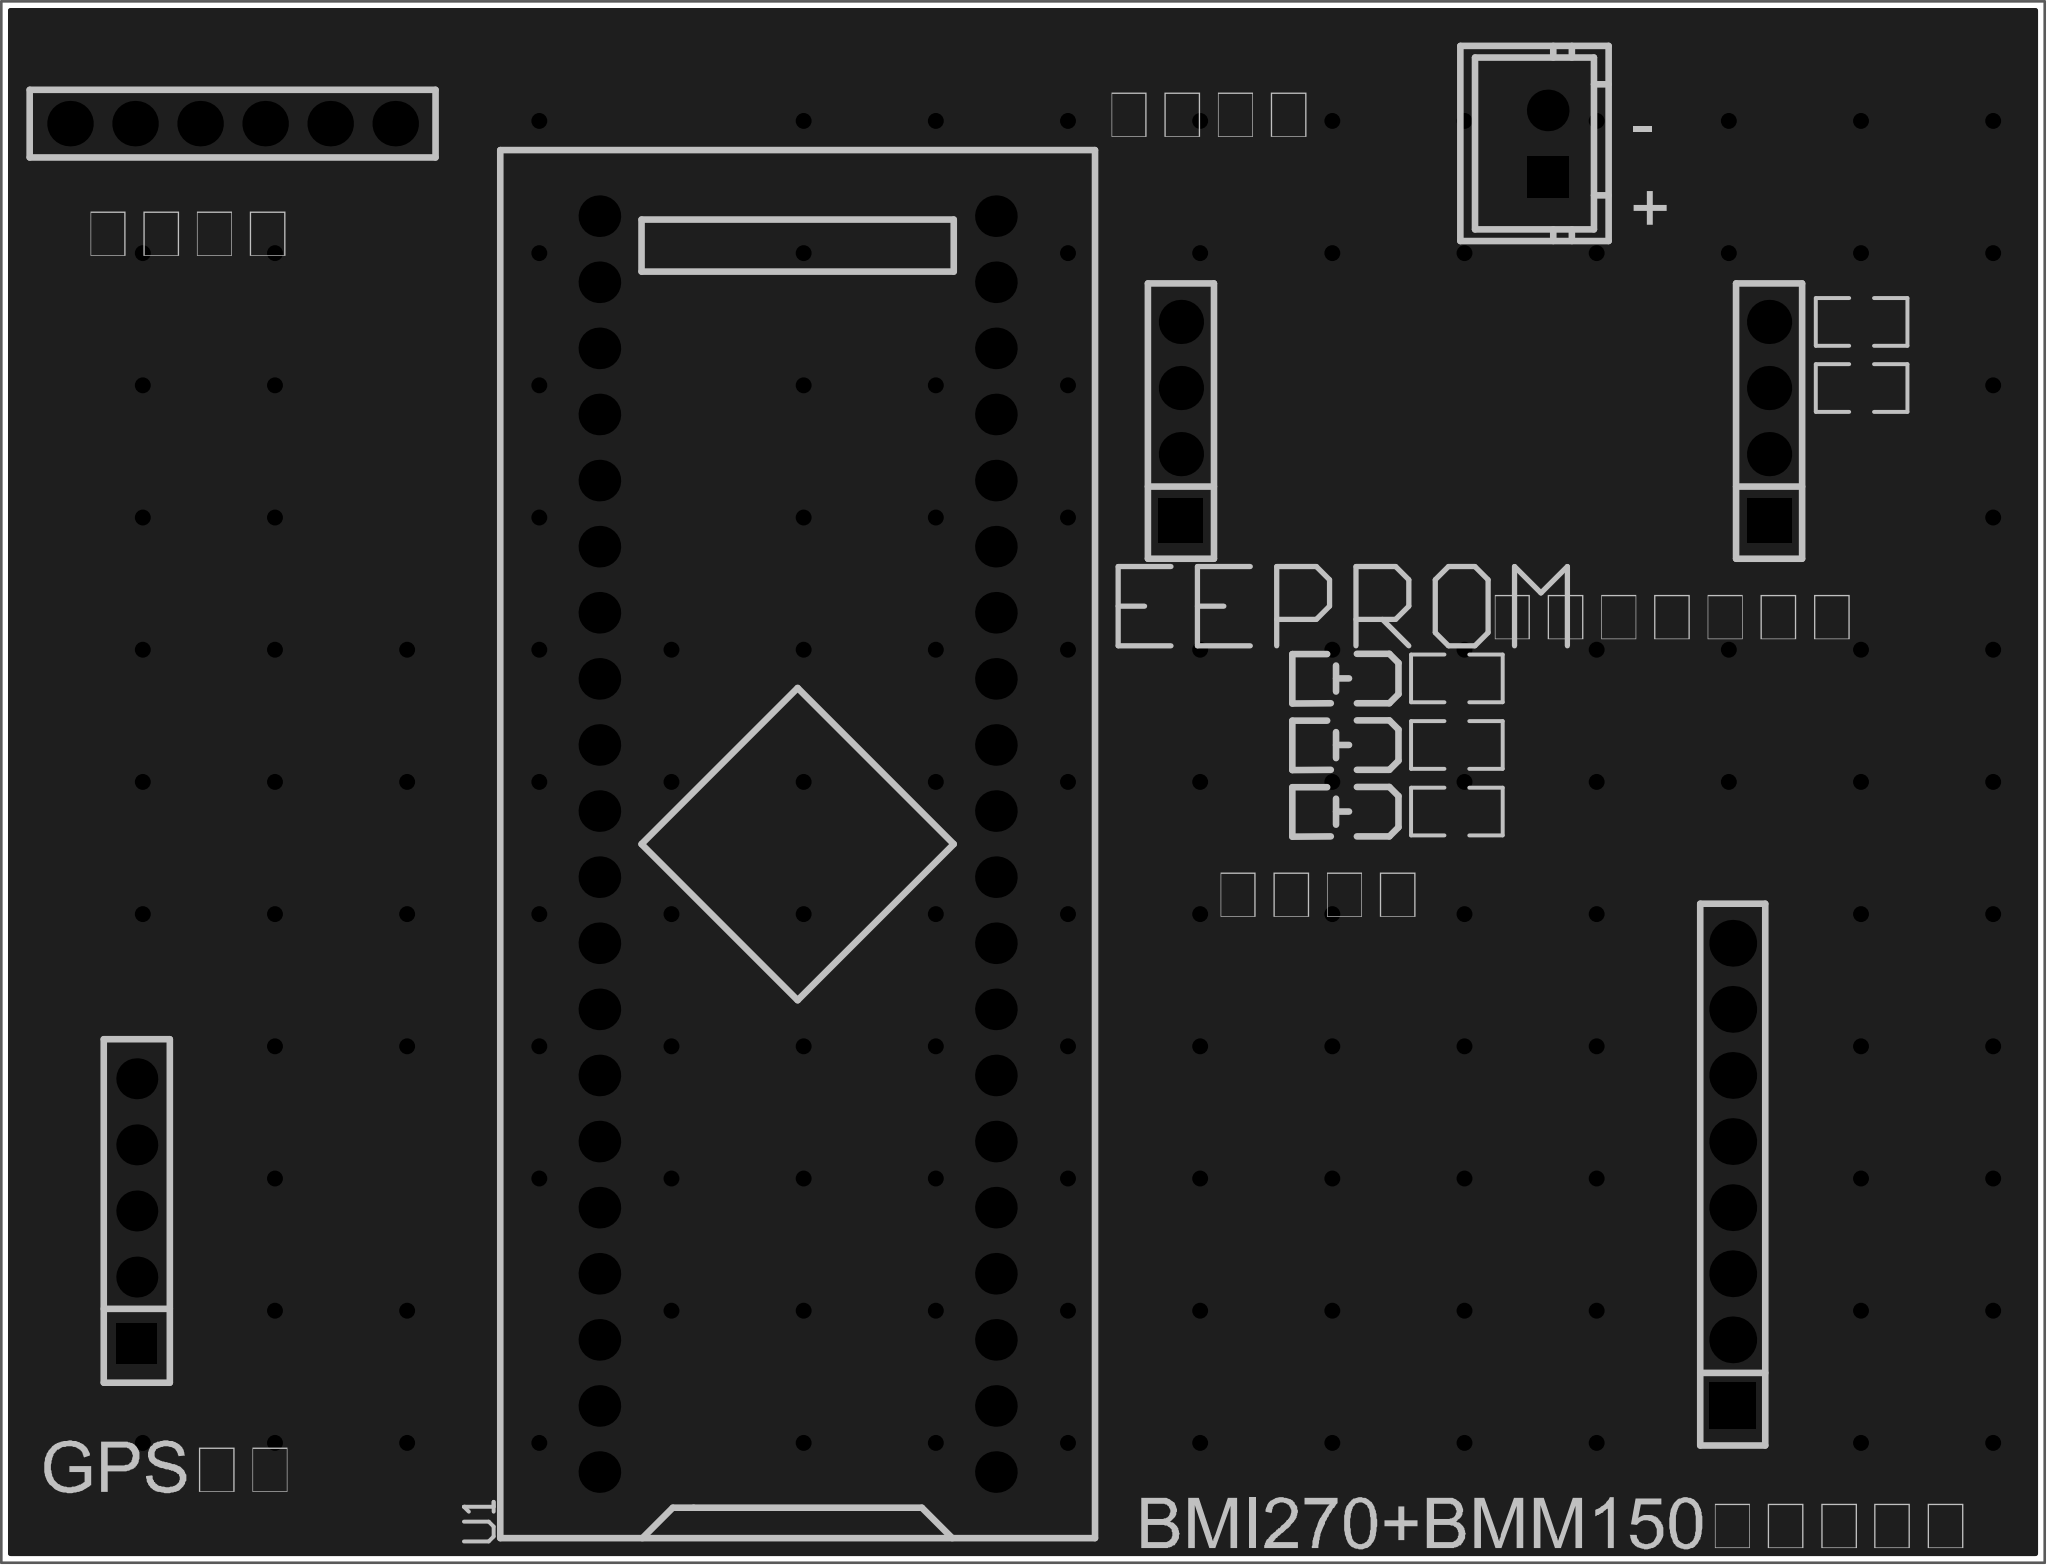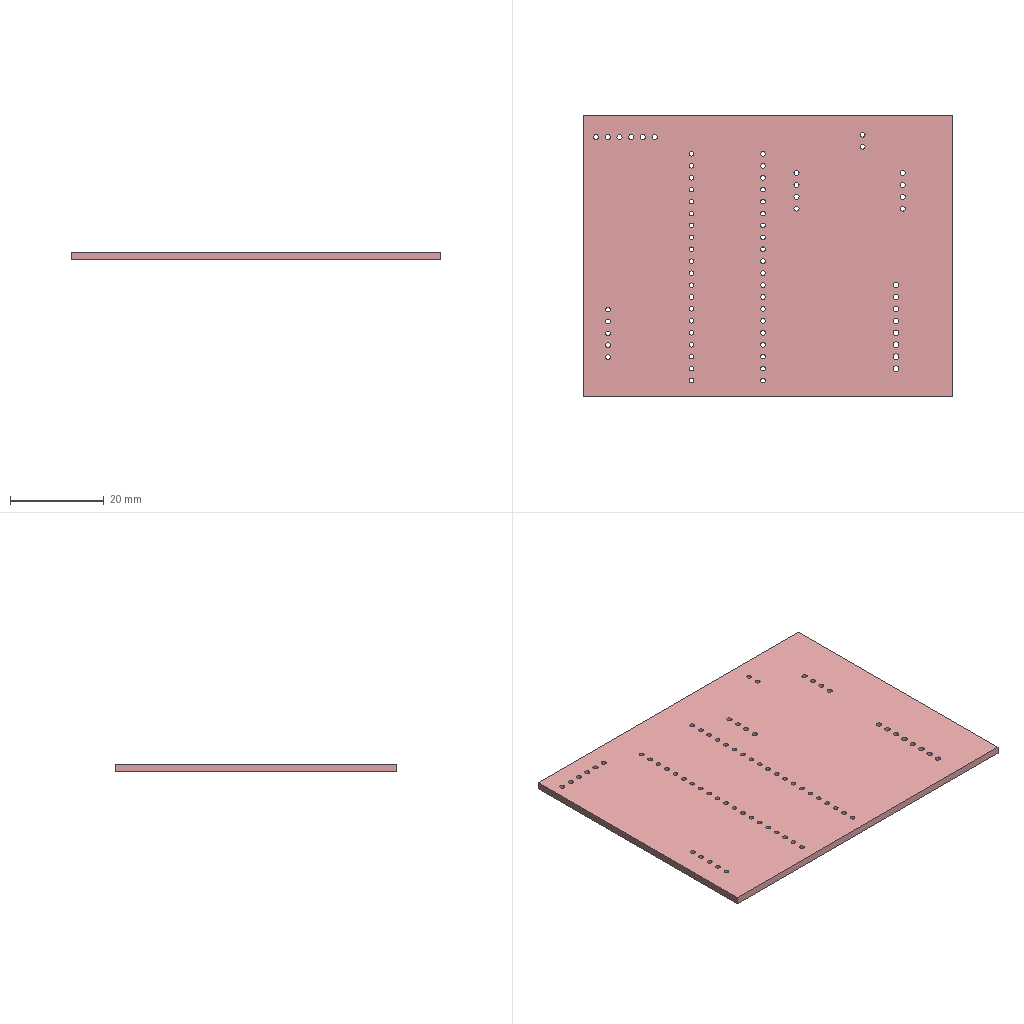Circuit board layout | Altium Designer | box 78.5 x 60 x 1.6 mm
Layer stack:
# Altium Designer layer stack of  (unit mm; dielectric type: 0 none, 1 core, 2 prepreg, 3 surface material)
index,name,kind,layer,copper_thickness_mm,dielectric_type,dielectric_thickness_mm,dielectric_material,dielectric_constant
0,Top Paste Mask Layer,other,,,,,,
1,Top Silkscreen Layer,other,,,,,,
2,Top Solder Mask Layer,dielectric,,,3,0.01,,3.3
3,Top Layer,copper,Top Layer,0.035,,,,
4,Dielectric1,dielectric,,,3,1.51,FR4,4.5
5,Bottom Layer,copper,Bottom Layer,0.035,,,,
6,Bottom Solder Mask Layer,dielectric,,,3,0.01,,3.3
7,Bottom Silkscreen Layer,other,,,,,,
8,Bottom Paste Mask Layer,other,,,,,,
# drill layer pairs: low layer,high layer
drill_pair,Top Layer,Bottom Layer
Part placement:
Designator,Comment,Layer,Footprint,Center-X(mm),Center-Y(mm),Rotation
H4,,TopLayer,HDR-TH_4P-P2.54-V-F,124.333,123.317,90
H5,,TopLayer,HDR-TH_4P-P2.54-V-F,146.939,123.317,90
H6,,TopLayer,HDR-TH_8P-P2.54-V-F-1,145.542,94.361,90
U1,STM32F103C8T6-Card,TopLayer,CONN-TH_L53.3-W22.9_STM32F103C8T6-CARD,109.601,107.061,90
U2,_x001F_XH2.54-2P,TopLayer,CONN-TH_2P-P2.54-V,138.43,133.985,90
U3,HC-05_排母*6P,TopLayer,HDR-TH_6P-P2.50-V-F-R1-C6,87.884,134.747,0
LED1,,TopLayer,LED_0805,130.595,108.307,180
LED2,,TopLayer,LED_0805,130.595,110.865,180
LED3,,TopLayer,LED_0805,130.595,113.423,180
R4,4.7K,TopLayer,R0805,150.495,124.587,180
R5,4.7K,TopLayer,R0805,150.495,127.127,180
R6,4.7K,TopLayer,R0805,134.939,108.312,0
R7,4.7K,TopLayer,R0805,134.939,110.87,0
R8,4.7K,TopLayer,R0805,134.939,113.429,0
H7,,TopLayer,HDR-TH_5P-P2.54-V-F,84.201,92.964,90
Pad and via stacks:
# Altium Designer via and pad stacks of  (unit mm). Each distinct definition once, with the count of objects using it.
# via: kind,start_layer,end_layer,hole_mm,diameter_mm,mode(0 simple;1 top-mid-bottom;2 full stack),diameter_per_layer,count,example_net
# pad: kind,layer,hole_mm,hole_type(0 round;1 square;2 slot),plating,top_size,top_shape(1 round;2 rect;3 octagon;9 rounded rect),mid_size,bottom_size,mode,footprint,size_per_layer,count,example
pad,Multi-Layer,1.1,0,plated,1.7x1.7,2,1.7x1.7,1.7x1.7,0,HDR-TH_4P-P2.54-V-F,,2,H4.1
pad,Multi-Layer,1.1,0,plated,1.7x1.7,1,1.7x1.7,1.7x1.7,0,HDR-TH_4P-P2.54-V-F,,6,H4.2
pad,Multi-Layer,1.2,0,plated,1.8x1.8,2,1.8x1.8,1.8x1.8,0,HDR-TH_8P-P2.54-V-F-1,,1,H6.1
pad,Multi-Layer,1.2,0,plated,1.8x1.8,1,1.8x1.8,1.8x1.8,0,HDR-TH_8P-P2.54-V-F-1,,7,H6.2
pad,Multi-Layer,1,0,plated,1.6x1.6,1,1.6x1.6,1.6x1.6,0,CONN-TH_L53.3-W22.9_STM32F103C8T6-CARD,,40,U1.1
pad,Multi-Layer,1,0,plated,1.6x1.6,1,1.6x1.6,1.6x1.6,0,CONN-TH_2P-P2.54-V,,1,U2.2
pad,Multi-Layer,1,0,plated,1.6x1.6,2,1.6x1.6,1.6x1.6,0,CONN-TH_2P-P2.54-V,,1,U2.1
pad,Multi-Layer,1.1,0,plated,1.75x1.75,1,1.75x1.75,1.75x1.75,0,HDR-TH_6P-P2.50-V-F-R1-C6,,6,U3.1
pad,Multi-Layer,1.02,0,plated,1.575x1.575,1,1.575x1.575,1.575x1.575,0,HDR-TH_5P-P2.54-V-F,,4,H7.5
pad,Multi-Layer,1.02,0,plated,1.575x1.575,2,1.575x1.575,1.575x1.575,0,HDR-TH_5P-P2.54-V-F,,1,H7.1
pad,Top Layer,0,0,plated,1x1.25,2,1x1.25,1x1.25,0,LED_0805,,6,LED1.2
pad,Top Layer,0,0,plated,1.133x1.377,2,1.133x1.377,1.133x1.377,0,R0805,,10,R4.2
via,Top Layer,Bottom Layer,0.3048,0.61,0,,131,GND
Copper pours:
name,layer,net,type(0 solid;1 hatched;2 none)
Top Layer-GND,Top Layer,GND,0
Bottom Layer-GND,Bottom Layer,GND,0